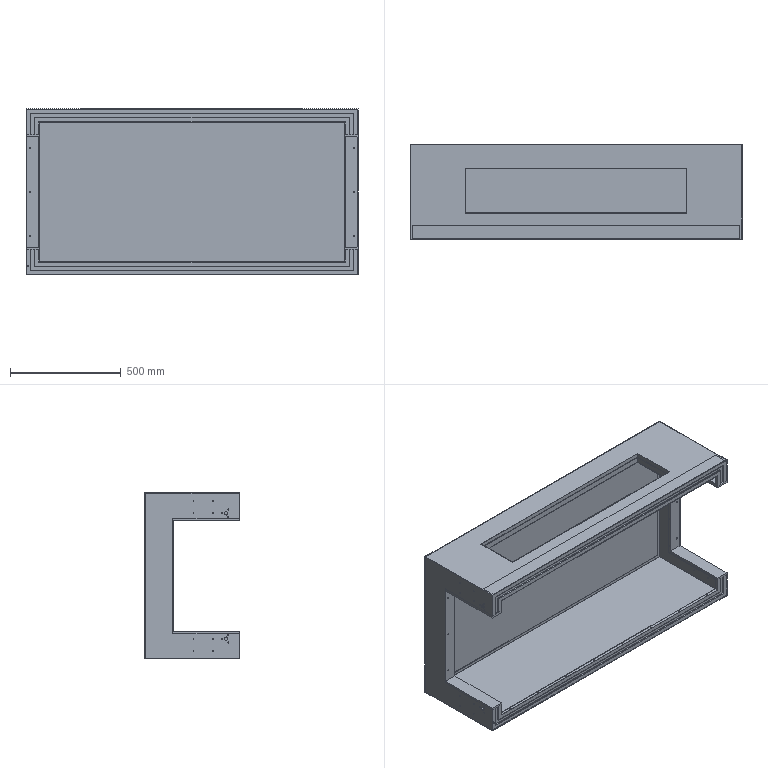Part | STEP file | 2 solids | 322 faces | box 1500 x 430 x 750 mm | volume 6110205 mm3 | cylinder 194 | plane 128 | commonest cylinder face diameters 4.5 x120 4 x32 5 x24 8 x12 15 x4 7 x2